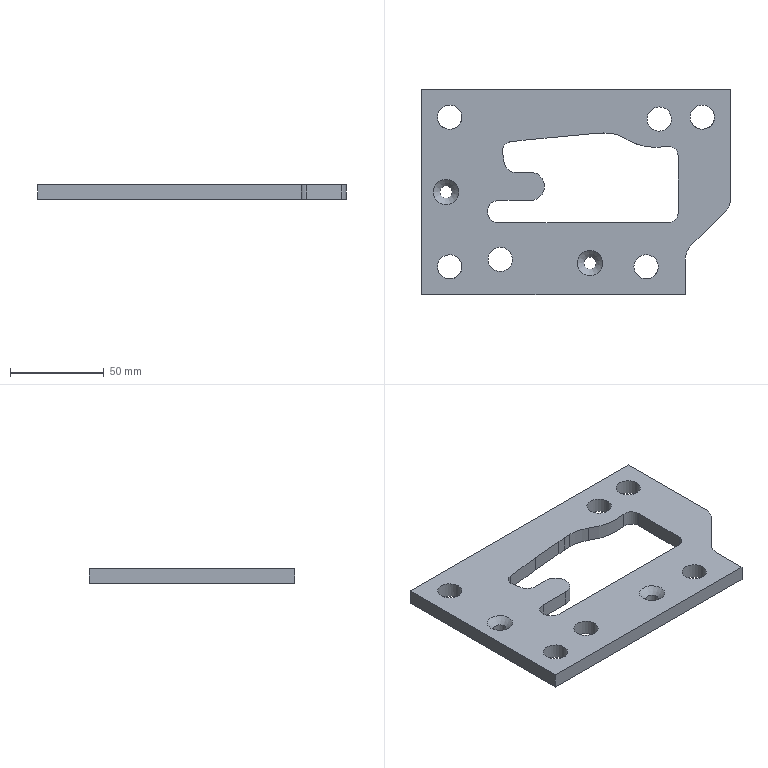Part | STEP file | gslz 2016.10.28-13_id146_x_t | 1 solid | 38 faces | box 165 x 110 x 8 mm | volume 99840 mm3 | cylinder 20 | plane 16 | cone 2 | commonest cylinder face diameters 13 x6 10 x3 12 x3 6.5 x2 15 x1 18 x1